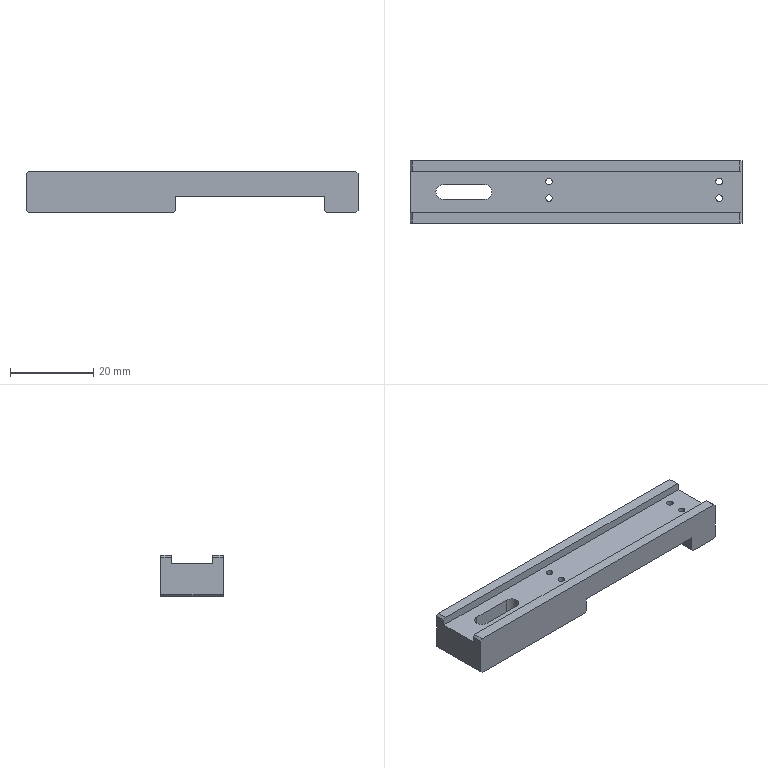NC program | NX | posted with a generic post | part box 80 x 15 x 10 mm
Whole program:
N10 G17 G21 G94 G90
(FLOOR_WALL_COPY , TOOL : D63)
N12 T03 M6
N14 G54
N16 G17 G0 G90 X-74.5 Y0. S6500 M3
N18 G43 Z30. H3
N20 Z7.
N22 G94 G1 Z4. F1500.
N24 X-71.5
N26 X71.5
N28 X74.5
N30 Z7.
N32 G0 Z30.
N34 X-74.5
N36 Z6.
N38 G1 Z3.
N40 X-71.5
N42 X71.5
N44 X74.5
N46 Z6.
N48 G0 Z30.
N50 X-74.5
N52 Z5.
N54 G1 Z2.
N56 X-71.5
N58 X71.5
N60 X74.5
N62 Z5.
N64 G0 Z30.
N66 X-74.5
N68 Z4.
N70 G1 Z1.
N72 X-71.5
N74 X71.5
N76 X74.5
N78 Z4.
N80 G0 Z30.
N82 X-74.5
N84 Z3.
N86 G1 Z0.
N88 X-71.5
N90 X71.5
N92 X74.5
N94 Z3.
N96 G0 Z30.
N98 M5
(ZLEVEL_PROFILE_1_COPY_COPY , TOOL : D6)
N100 T16 M6
N102 G54
N104 G17 G0 G90 X-48.969 Y-1.13 S7500 M3
N106 G43 Z30. H16
N108 Z0.4
N110 G94 G1 X-48.961 Y-1.141 Z0.263 F1000.
N112 X-48.934 Y-1.172 Z0.14
N114 X-48.887 Y-1.22 Z0.03
N116 X-48.818 Y-1.281 Z-0.068
N118 X-48.725 Y-1.353 Z-0.153
N120 X-48.604 Y-1.431 Z-0.228
N122 X-48.455 Y-1.513 Z-0.292
N124 X-48.276 Y-1.595 Z-0.346
N126 X-48.063 Y-1.674 Z-0.391
N128 X-47.814 Y-1.747 Z-0.427
N130 X-47.529 Y-1.81 Z-0.455
N132 X-47.204 Y-1.861 Z-0.476
N134 X-46.838 Y-1.895 Z-0.49
N136 X-46.428 Y-1.909 Z-0.497
N138 X-45.972 Y-1.901 Z-0.5
N140 X-45.946 Y-1.9 F1650.
N142 X-39.609
N144 X39.98
N146 X45.946
N148 X45.972 Y-1.901
N150 X46.219 Y-1.897
N152 X46.444 Y-1.863
N154 X46.648 Y-1.803
N156 X46.831 Y-1.72
N158 X46.995 Y-1.617
N160 X47.141 Y-1.499
N162 X47.269 Y-1.368
N164 X47.382 Y-1.227
N166 X47.479 Y-1.08
N168 X47.563 Y-0.93
N170 X47.634 Y-0.78
N172 X47.733 Y-0.513
N174 X47.792 Y-0.254
N176 X47.812 Y0.
N178 X47.792 Y0.254
N180 X47.733 Y0.513
N182 X47.634 Y0.78
N184 X47.563 Y0.93
N186 X47.479 Y1.08
N188 X47.382 Y1.227
N190 X47.269 Y1.368
N192 X47.141 Y1.499
N194 X46.995 Y1.617
N196 X46.831 Y1.72
N198 X46.648 Y1.803
N200 X46.444 Y1.863
N202 X46.219 Y1.897
N204 X45.972 Y1.901
N206 X45.946 Y1.9
N208 X40.
N210 X-39.609
N212 X-45.946
N214 X-45.972 Y1.901
N216 X-46.221 Y1.897 Z-0.502
N218 X-46.448 Y1.863 Z-0.506
N220 X-46.654 Y1.803 Z-0.513
N222 X-46.838 Y1.72 Z-0.522
N224 X-47.004 Y1.617 Z-0.534
N226 X-47.151 Y1.499 Z-0.547
N228 X-47.281 Y1.367 Z-0.563
N230 X-47.395 Y1.226 Z-0.579
N232 X-47.493 Y1.079 Z-0.597
N234 X-47.578 Y0.929 Z-0.616
N236 X-47.649 Y0.779 Z-0.635
N238 X-47.749 Y0.513 Z-0.673
N240 X-47.81 Y0.254 Z-0.711
N242 X-47.83 Y0. Z-0.75
N244 X-47.81 Y-0.254 Z-0.789
N246 X-47.751 Y-0.512 Z-0.827
N248 X-47.651 Y-0.779 Z-0.865
N250 X-47.58 Y-0.928 Z-0.884
N252 X-47.496 Y-1.079 Z-0.903
N254 X-47.398 Y-1.226 Z-0.921
N256 X-47.284 Y-1.367 Z-0.937
N258 X-47.155 Y-1.498 Z-0.953
N260 X-47.008 Y-1.617 Z-0.966
N262 X-46.843 Y-1.719 Z-0.978
N264 X-46.658 Y-1.802 Z-0.987
N266 X-46.453 Y-1.862 Z-0.994
N268 X-46.226 Y-1.896 Z-0.998
N270 X-45.977 Y-1.901 Z-1.
N272 X-45.946 Y-1.9
N274 X-39.961
N276 X-39.609
N278 X40. Y-1.899
N280 X40.344 Y-1.919
N282 X40.357 Y-1.899
N284 X45.946 Y-1.9
N286 X45.977 Y-1.901
N288 X46.224 Y-1.896
N290 X46.449 Y-1.862
N292 X46.652 Y-1.802
N294 X46.836 Y-1.719
N296 X46.999 Y-1.617
N298 X47.145 Y-1.499
N300 X47.274 Y-1.367
N302 X47.386 Y-1.226
N304 X47.484 Y-1.079
N306 X47.568 Y-0.929
N308 X47.638 Y-0.78
N310 X47.737 Y-0.513
N312 X47.797 Y-0.254
N314 X47.816 Y0.
N316 X47.797 Y0.254
N318 X47.737 Y0.513
N320 X47.638 Y0.78
N322 X47.568 Y0.929
N324 X47.484 Y1.079
N326 X47.386 Y1.226
N328 X47.274 Y1.367
N330 X47.145 Y1.499
N332 X46.999 Y1.617
N334 X46.836 Y1.719
N336 X46.652 Y1.802
N338 X46.449 Y1.862
N340 X46.224 Y1.896
N342 X45.977 Y1.901
N344 X45.946 Y1.9
N346 X40.357 Y1.899
N348 X40. Y1.9
N350 X-39.609
N352 X-40.313 Y1.899
N354 X-45.946 Y1.9
N356 X-45.977 Y1.901
N358 X-46.226 Y1.896 Z-1.002
N360 X-46.453 Y1.862 Z-1.006
N362 X-46.658 Y1.802 Z-1.013
N364 X-46.843 Y1.719 Z-1.022
N366 X-47.009 Y1.617 Z-1.034
N368 X-47.156 Y1.498 Z-1.047
N370 X-47.285 Y1.367 Z-1.063
N372 X-47.399 Y1.226 Z-1.079
N374 X-47.498 Y1.079 Z-1.097
N376 X-47.582 Y0.929 Z-1.116
N378 X-47.654 Y0.779 Z-1.135
N380 X-47.754 Y0.512 Z-1.173
N382 X-47.814 Y0.254 Z-1.211
N384 X-47.835 Y0. Z-1.25
N386 X-47.815 Y-0.254 Z-1.289
N388 X-47.755 Y-0.512 Z-1.327
N390 X-47.656 Y-0.779 Z-1.365
N392 X-47.585 Y-0.928 Z-1.384
N394 X-47.501 Y-1.078 Z-1.403
N396 X-47.402 Y-1.226 Z-1.421
N398 X-47.289 Y-1.367 Z-1.437
N400 X-47.16 Y-1.498 Z-1.453
N402 X-47.013 Y-1.617 Z-1.466
N404 X-46.847 Y-1.719 Z-1.478
N406 X-46.663 Y-1.802 Z-1.487
N408 X-46.458 Y-1.862 Z-1.494
N410 X-46.231 Y-1.896 Z-1.498
N412 X-45.981 Y-1.901 Z-1.5
N414 X-45.946 Y-1.899
N416 X-39.961 Y-1.9
N418 X-39.609
N420 X39.98
N422 X40. Y-1.899
N424 X40.333 Y-1.918
N426 X40.346 Y-1.899
N428 X45.946
N430 X45.981 Y-1.901
N432 X46.229 Y-1.896
N434 X46.454 Y-1.862
N436 X46.657 Y-1.802
N438 X46.84 Y-1.719
N440 X47.004 Y-1.617
N442 X47.15 Y-1.498
N444 X47.278 Y-1.367
N446 X47.391 Y-1.226
N448 X47.489 Y-1.079
N450 X47.572 Y-0.929
N452 X47.643 Y-0.779
N454 X47.742 Y-0.513
N456 X47.801 Y-0.254
N458 X47.821 Y0.
N460 X47.801 Y0.254
N462 X47.742 Y0.513
N464 X47.643 Y0.779
N466 X47.572 Y0.929
N468 X47.489 Y1.079
N470 X47.391 Y1.226
N472 X47.278 Y1.367
N474 X47.15 Y1.498
N476 X47.004 Y1.617
N478 X46.84 Y1.719
N480 X46.657 Y1.802
N482 X46.454 Y1.862
N484 X46.229 Y1.896
N486 X45.981 Y1.901
N488 X45.946 Y1.899
N490 X40.346
N492 X40. Y1.9
N494 X-39.609
N496 X-40.313 Y1.899
N498 X-45.946
N500 X-45.981 Y1.901
N502 X-46.231 Y1.896 Z-1.502
N504 X-46.458 Y1.862 Z-1.506
N506 X-46.663 Y1.802 Z-1.513
N508 X-46.848 Y1.719 Z-1.522
N510 X-47.013 Y1.617 Z-1.534
N512 X-47.16 Y1.498 Z-1.547
N514 X-47.29 Y1.367 Z-1.563
N516 X-47.404 Y1.226 Z-1.579
N518 X-47.502 Y1.079 Z-1.597
N520 X-47.587 Y0.928 Z-1.616
N522 X-47.658 Y0.779 Z-1.635
N524 X-47.759 Y0.512 Z-1.673
N526 X-47.819 Y0.254 Z-1.711
N528 X-47.839 Y0. Z-1.75
N530 X-47.82 Y-0.254 Z-1.789
N532 X-47.76 Y-0.512 Z-1.827
N534 X-47.661 Y-0.778 Z-1.865
N536 X-47.589 Y-0.928 Z-1.884
N538 X-47.505 Y-1.078 Z-1.903
N540 X-47.407 Y-1.225 Z-1.921
N542 X-47.294 Y-1.366 Z-1.937
N544 X-47.164 Y-1.498 Z-1.953
N546 X-47.017 Y-1.616 Z-1.966
N548 X-46.852 Y-1.719 Z-1.978
N550 X-46.668 Y-1.802 Z-1.987
N552 X-46.462 Y-1.862 Z-1.994
N554 X-46.236 Y-1.896 Z-1.998
N556 X-45.986 Y-1.9 Z-2.
N558 X-45.946 Y-1.899
N560 X-40.313
N562 X-39.609 Y-1.9
N564 X39.98
N566 X40. Y-1.899
N568 X40.333 Y-1.918
N570 X40.346 Y-1.899
N572 X45.946
N574 X45.986 Y-1.9
N576 X46.233 Y-1.896
N578 X46.458 Y-1.863
N580 X46.662 Y-1.804
N582 X46.845 Y-1.722
N584 X47.009 Y-1.622
N586 X47.155 Y-1.506
N588 X47.283 Y-1.377
N590 X47.396 Y-1.239
N592 X47.493 Y-1.095
N594 X47.577 Y-0.948
N596 X47.648 Y-0.801
N598 X47.747 Y-0.541
N600 X47.806 Y-0.288
N602 X47.826 Y-0.039
N604 X47.807 Y0.21
N606 X47.747 Y0.466
N608 X47.649 Y0.73
N610 X47.578 Y0.88
N612 X47.494 Y1.03
N614 X47.397 Y1.179
N616 X47.284 Y1.322
N618 X47.155 Y1.456
N620 X47.01 Y1.578
N622 X46.846 Y1.686
N624 X46.662 Y1.775
N626 X46.459 Y1.843
N628 X46.234 Y1.885
N630 X45.986 Y1.9
N632 X40.
N634 X-39.609
N636 X-40.313 Y1.899
N638 X-45.946
N640 X-45.986 Y1.9
N642 X-46.442 Y1.908 Z-1.997
N644 X-46.852 Y1.894 Z-1.99
N646 X-47.219 Y1.86 Z-1.976
N648 X-47.543 Y1.809 Z-1.955
N650 X-47.829 Y1.746 Z-1.927
N652 X-48.077 Y1.673 Z-1.891
N654 X-48.29 Y1.594 Z-1.846
N656 X-48.47 Y1.512 Z-1.792
N658 X-48.619 Y1.43 Z-1.728
N660 X-48.739 Y1.352 Z-1.653
N662 X-48.833 Y1.28 Z-1.568
N664 X-48.902 Y1.219 Z-1.47
N666 X-48.949 Y1.171 Z-1.36
N668 X-48.975 Y1.14 Z-1.237
N670 X-48.983 Y1.129 Z-1.1
N672 G0 Z30.
N674 M5
(PLANAR_MILL_COPY_1 , TOOL : D6A45)
N676 T01 M6
N678 G54
N680 G17 G0 G90 X-0.766 Y8.757 S7500 M3
N682 G43 Z30. H1
N684 Z1.
N686 G94 G1 Z-1. F1250.
N688 G3 X0. Y8.4 R1.
N690 G1 X40.
N692 G2 X40.9 Y7.5 R0.9
N694 G1 Y5.
N696 G2 X40. Y4.1 R0.9
N698 G1 X-40.
N700 G2 X-40.9 Y5. R0.9
N702 G1 Y7.5
N704 G2 X-40. Y8.4 R0.9
N706 G1 X0.
N708 G3 X0.766 Y8.757 R1.
N710 G1 Z1.
N712 G0 Z30.
N714 Y-8.757
N716 Z1.
N718 G1 Z-1.
N720 G3 X0. Y-8.4 R1.
N722 G1 X-40.
N724 G2 X-40.9 Y-7.5 R0.9
N726 G1 Y-5.
N728 G2 X-40. Y-4.1 R0.9
N730 G1 X40.
N732 G2 X40.9 Y-5. R0.9
N734 G1 Y-7.5
N736 G2 X40. Y-8.4 R0.9
N738 G1 X0.
N740 G3 X-0.766 Y-8.757 R1.
N742 G1 Z1.
N744 G0 Z30.
N746 M5
(刀补16 , TOOL : D6)
N748 T16 M6
N750 G54
N752 G17 G0 G90 X44.325 Y0.776 S7500 M3
N754 G43 Z30. H16
N756 Z1.
N758 G94 G1 Z-2. F1000.
N760 G41 X44.29 Y0.869 D16
N762 X43.822 Y1.657
N764 G3 X43.299 Y1.951 R0.6
N766 G1 X43.112 Y1.949
N768 X40. Y1.95
N770 X-40.
N772 X-43.112 Y1.949
N774 X-43.299 Y1.951
N776 G3 X-43.822 Y1.657 R0.6
N778 G1 X-44.289 Y0.869
N780 G40
N782 X-44.325 Y0.775
N784 Z1.
N786 G0 Z30.
N788 X-44.326 Y-0.773
N790 Z1.
N792 G1 Z-2.
N794 G41 X-44.291 Y-0.866
N796 X-43.822 Y-1.657
N798 G3 X-43.299 Y-1.951 R0.6
N800 G1 X-43.112 Y-1.949
N802 X-39.621 Y-1.95
N804 X39.985
N806 X40. Y-1.949
N808 X40.329 Y-1.968
N810 X40.341 Y-1.949
N812 X43.112
N814 X43.299 Y-1.951
N816 G3 X43.822 Y-1.657 R0.6
N818 G1 X44.29 Y-0.868
N820 G40
N822 X44.326 Y-0.774
N824 Z1.
N826 G0 Z30.
N828 M5
N830 M2